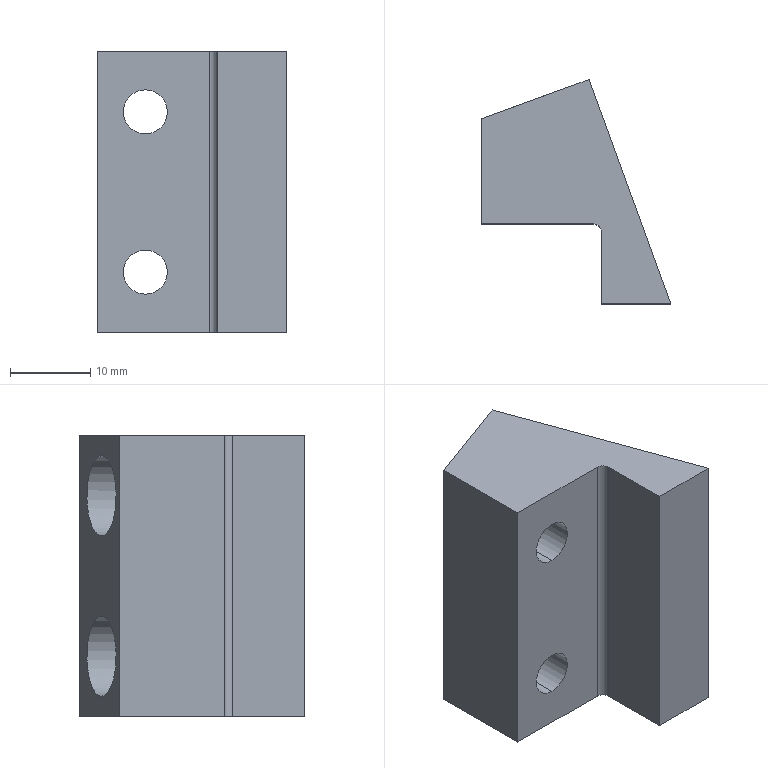Part | SolidWorks | features BaseBody 1 | 1 solid | 19 faces | box 23.64 x 28 x 35 mm | volume 9816 mm3 | plane 10 | cylinder 9 | commonest cylinder face diameters 5.5 x4 10 x4 2 x1
STEP:
#1=CARTESIAN_POINT('',(6.,4.,2.5));
#2=VERTEX_POINT('',#1);
#3=CARTESIAN_POINT('',(6.,4.,12.5));
#4=VERTEX_POINT('',#3);
#5=CARTESIAN_POINT('',(6.,4.,7.5));
#6=DIRECTION('',(0.,1.,0.));
#7=DIRECTION('',(0.,0.,1.));
#8=AXIS2_PLACEMENT_3D('',#5,#6,#7);
#9=CIRCLE('',#8,5.);
#10=EDGE_CURVE('',#2,#4,#9,.T.);
#11=ORIENTED_EDGE('',*,*,#10,.F.);
#12=CARTESIAN_POINT('',(6.,15.289,2.5));
#13=VERTEX_POINT('',#12);
#14=CARTESIAN_POINT('',(6.,18.,2.5));
#15=DIRECTION('',(0.,1.,0.));
#16=VECTOR('',#15,1000.);
#17=LINE('',#14,#16);
#18=EDGE_CURVE('',#2,#13,#17,.T.);
#19=ORIENTED_EDGE('',*,*,#18,.T.);
#20=CARTESIAN_POINT('',(6.,15.289,12.5));
#21=VERTEX_POINT('',#20);
#22=CARTESIAN_POINT('',(6.,15.289,2.5));
#23=CARTESIAN_POINT('',(-4.,11.649,2.5));
#24=CARTESIAN_POINT('',(-4.,11.649,12.5));
#25=CARTESIAN_POINT('',(6.,15.289,12.5));
#26=(BOUNDED_CURVE()B_SPLINE_CURVE(3,(#22,#23,#24,#25),.UNSPECIFIED.,.F.,.F.)B_SPLINE_CURVE_WITH_KNOTS((4,4),(1.571,4.712),.UNSPECIFIED.)CURVE()GEOMETRIC_REPRESENTATION_ITEM()RATIONAL_B_SPLINE_CURVE((1.,0.3333,0.3333,1.))REPRESENTATION_ITEM(''));
#27=EDGE_CURVE('',#13,#21,#26,.T.);
#28=ORIENTED_EDGE('',*,*,#27,.T.);
#29=CARTESIAN_POINT('',(6.,18.,12.5));
#30=DIRECTION('',(0.,1.,0.));
#31=VECTOR('',#30,1000.);
#32=LINE('',#29,#31);
#33=EDGE_CURVE('',#4,#21,#32,.T.);
#34=ORIENTED_EDGE('',*,*,#33,.F.);
#35=EDGE_LOOP('',(#11,#19,#28,#34));
#36=FACE_OUTER_BOUND('',#35,.T.);
#37=CARTESIAN_POINT('',(6.,18.,7.5));
#38=DIRECTION('',(0.,1.,0.));
#39=DIRECTION('',(0.,0.,1.));
#40=AXIS2_PLACEMENT_3D('',#37,#38,#39);
#41=CYLINDRICAL_SURFACE('',#40,5.);
#42=ADVANCED_FACE('',(#36),#41,.F.);
#43=CARTESIAN_POINT('',(6.,4.,22.5));
#44=VERTEX_POINT('',#43);
#45=CARTESIAN_POINT('',(6.,4.,32.5));
#46=VERTEX_POINT('',#45);
#47=CARTESIAN_POINT('',(6.,4.,27.5));
#48=DIRECTION('',(0.,1.,0.));
#49=DIRECTION('',(0.,0.,1.));
#50=AXIS2_PLACEMENT_3D('',#47,#48,#49);
#51=CIRCLE('',#50,5.);
#52=EDGE_CURVE('',#44,#46,#51,.T.);
#53=ORIENTED_EDGE('',*,*,#52,.F.);
#54=CARTESIAN_POINT('',(6.,15.289,22.5));
#55=VERTEX_POINT('',#54);
#56=CARTESIAN_POINT('',(6.,18.,22.5));
#57=DIRECTION('',(0.,1.,0.));
#58=VECTOR('',#57,1000.);
#59=LINE('',#56,#58);
#60=EDGE_CURVE('',#44,#55,#59,.T.);
#61=ORIENTED_EDGE('',*,*,#60,.T.);
#62=CARTESIAN_POINT('',(6.,15.289,32.5));
#63=VERTEX_POINT('',#62);
#64=CARTESIAN_POINT('',(6.,15.289,22.5));
#65=CARTESIAN_POINT('',(-4.,11.649,22.5));
#66=CARTESIAN_POINT('',(-4.,11.649,32.5));
#67=CARTESIAN_POINT('',(6.,15.289,32.5));
#68=(BOUNDED_CURVE()B_SPLINE_CURVE(3,(#64,#65,#66,#67),.UNSPECIFIED.,.F.,.T.)B_SPLINE_CURVE_WITH_KNOTS((4,4),(1.571,4.712),.UNSPECIFIED.)CURVE()GEOMETRIC_REPRESENTATION_ITEM()RATIONAL_B_SPLINE_CURVE((1.,0.3333,0.3333,1.))REPRESENTATION_ITEM(''));
#69=EDGE_CURVE('',#55,#63,#68,.T.);
#70=ORIENTED_EDGE('',*,*,#69,.T.);
#71=CARTESIAN_POINT('',(6.,18.,32.5));
#72=DIRECTION('',(0.,1.,0.));
#73=VECTOR('',#72,1000.);
#74=LINE('',#71,#73);
#75=EDGE_CURVE('',#46,#63,#74,.T.);
#76=ORIENTED_EDGE('',*,*,#75,.F.);
#77=EDGE_LOOP('',(#53,#61,#70,#76));
#78=FACE_OUTER_BOUND('',#77,.T.);
#79=CARTESIAN_POINT('',(6.,18.,27.5));
#80=DIRECTION('',(0.,1.,0.));
#81=DIRECTION('',(0.,0.,1.));
#82=AXIS2_PLACEMENT_3D('',#79,#80,#81);
#83=CYLINDRICAL_SURFACE('',#82,5.);
#84=ADVANCED_FACE('',(#78),#83,.F.);
#85=CARTESIAN_POINT('',(6.,0.,30.25));
#86=VERTEX_POINT('',#85);
#87=CARTESIAN_POINT('',(6.,0.,24.75));
#88=VERTEX_POINT('',#87);
#89=CARTESIAN_POINT('',(6.,0.,27.5));
#90=DIRECTION('',(0.,-1.,0.));
#91=DIRECTION('',(0.,0.,1.));
#92=AXIS2_PLACEMENT_3D('',#89,#90,#91);
#93=CIRCLE('',#92,2.75);
#94=EDGE_CURVE('',#86,#88,#93,.T.);
#95=ORIENTED_EDGE('',*,*,#94,.T.);
#96=CARTESIAN_POINT('',(6.,4.,24.75));
#97=VERTEX_POINT('',#96);
#98=CARTESIAN_POINT('',(6.,18.,24.75));
#99=DIRECTION('',(0.,1.,0.));
#100=VECTOR('',#99,1000.);
#101=LINE('',#98,#100);
#102=EDGE_CURVE('',#88,#97,#101,.T.);
#103=ORIENTED_EDGE('',*,*,#102,.T.);
#104=CARTESIAN_POINT('',(6.,4.,30.25));
#105=VERTEX_POINT('',#104);
#106=CARTESIAN_POINT('',(6.,4.,27.5));
#107=DIRECTION('',(0.,-1.,0.));
#108=DIRECTION('',(0.,0.,1.));
#109=AXIS2_PLACEMENT_3D('',#106,#107,#108);
#110=CIRCLE('',#109,2.75);
#111=EDGE_CURVE('',#105,#97,#110,.T.);
#112=ORIENTED_EDGE('',*,*,#111,.F.);
#113=CARTESIAN_POINT('',(6.,18.,30.25));
#114=DIRECTION('',(0.,1.,0.));
#115=VECTOR('',#114,1000.);
#116=LINE('',#113,#115);
#117=EDGE_CURVE('',#86,#105,#116,.T.);
#118=ORIENTED_EDGE('',*,*,#117,.F.);
#119=EDGE_LOOP('',(#95,#103,#112,#118));
#120=FACE_OUTER_BOUND('',#119,.T.);
#121=CARTESIAN_POINT('',(6.,18.,27.5));
#122=DIRECTION('',(0.,1.,0.));
#123=DIRECTION('',(0.,0.,1.));
#124=AXIS2_PLACEMENT_3D('',#121,#122,#123);
#125=CYLINDRICAL_SURFACE('',#124,2.75);
#126=ADVANCED_FACE('',(#120),#125,.F.);
#127=CARTESIAN_POINT('',(6.,0.,10.25));
#128=VERTEX_POINT('',#127);
#129=CARTESIAN_POINT('',(6.,0.,4.75));
#130=VERTEX_POINT('',#129);
#131=CARTESIAN_POINT('',(6.,0.,7.5));
#132=DIRECTION('',(0.,-1.,0.));
#133=DIRECTION('',(0.,0.,1.));
#134=AXIS2_PLACEMENT_3D('',#131,#132,#133);
#135=CIRCLE('',#134,2.75);
#136=EDGE_CURVE('',#128,#130,#135,.T.);
#137=ORIENTED_EDGE('',*,*,#136,.T.);
#138=CARTESIAN_POINT('',(6.,4.,4.75));
#139=VERTEX_POINT('',#138);
#140=CARTESIAN_POINT('',(6.,18.,4.75));
#141=DIRECTION('',(0.,1.,0.));
#142=VECTOR('',#141,1000.);
#143=LINE('',#140,#142);
#144=EDGE_CURVE('',#130,#139,#143,.T.);
#145=ORIENTED_EDGE('',*,*,#144,.T.);
#146=CARTESIAN_POINT('',(6.,4.,10.25));
#147=VERTEX_POINT('',#146);
#148=CARTESIAN_POINT('',(6.,4.,7.5));
#149=DIRECTION('',(0.,-1.,0.));
#150=DIRECTION('',(0.,0.,1.));
#151=AXIS2_PLACEMENT_3D('',#148,#149,#150);
#152=CIRCLE('',#151,2.75);
#153=EDGE_CURVE('',#147,#139,#152,.T.);
#154=ORIENTED_EDGE('',*,*,#153,.F.);
#155=CARTESIAN_POINT('',(6.,18.,10.25));
#156=DIRECTION('',(0.,1.,0.));
#157=VECTOR('',#156,1000.);
#158=LINE('',#155,#157);
#159=EDGE_CURVE('',#128,#147,#158,.T.);
#160=ORIENTED_EDGE('',*,*,#159,.F.);
#161=EDGE_LOOP('',(#137,#145,#154,#160));
#162=FACE_OUTER_BOUND('',#161,.T.);
#163=CARTESIAN_POINT('',(6.,18.,7.5));
#164=DIRECTION('',(0.,1.,0.));
#165=DIRECTION('',(0.,0.,1.));
#166=AXIS2_PLACEMENT_3D('',#163,#164,#165);
#167=CYLINDRICAL_SURFACE('',#166,2.75);
#168=ADVANCED_FACE('',(#162),#167,.F.);
#169=CARTESIAN_POINT('',(13.449,18.,35.));
#170=VERTEX_POINT('',#169);
#171=CARTESIAN_POINT('',(13.449,18.,0.));
#172=VERTEX_POINT('',#171);
#173=CARTESIAN_POINT('',(13.449,18.,35.));
#174=DIRECTION('',(0.,0.,-1.));
#175=VECTOR('',#174,1000.);
#176=LINE('',#173,#175);
#177=EDGE_CURVE('',#170,#172,#176,.T.);
#178=ORIENTED_EDGE('',*,*,#177,.F.);
#179=CARTESIAN_POINT('',(23.64,-10.,35.));
#180=VERTEX_POINT('',#179);
#181=CARTESIAN_POINT('',(13.449,18.,35.));
#182=DIRECTION('',(-0.342,0.9397,0.));
#183=VECTOR('',#182,1000.);
#184=LINE('',#181,#183);
#185=EDGE_CURVE('',#180,#170,#184,.T.);
#186=ORIENTED_EDGE('',*,*,#185,.F.);
#187=CARTESIAN_POINT('',(23.64,-10.,0.));
#188=VERTEX_POINT('',#187);
#189=CARTESIAN_POINT('',(23.64,-10.,35.));
#190=DIRECTION('',(0.,0.,1.));
#191=VECTOR('',#190,1000.);
#192=LINE('',#189,#191);
#193=EDGE_CURVE('',#188,#180,#192,.T.);
#194=ORIENTED_EDGE('',*,*,#193,.F.);
#195=CARTESIAN_POINT('',(13.449,18.,0.));
#196=DIRECTION('',(0.342,-0.9397,0.));
#197=VECTOR('',#196,1000.);
#198=LINE('',#195,#197);
#199=EDGE_CURVE('',#172,#188,#198,.T.);
#200=ORIENTED_EDGE('',*,*,#199,.F.);
#201=EDGE_LOOP('',(#178,#186,#194,#200));
#202=FACE_OUTER_BOUND('',#201,.T.);
#203=CARTESIAN_POINT('',(13.449,18.,35.));
#204=DIRECTION('',(-0.9397,-0.342,0.));
#205=DIRECTION('',(0.342,-0.9397,0.));
#206=AXIS2_PLACEMENT_3D('',#203,#204,#205);
#207=PLANE('',#206);
#208=ADVANCED_FACE('',(#202),#207,.F.);
#209=CARTESIAN_POINT('',(14.,0.,0.));
#210=VERTEX_POINT('',#209);
#211=CARTESIAN_POINT('',(0.,0.,0.));
#212=VERTEX_POINT('',#211);
#213=CARTESIAN_POINT('',(0.,0.,0.));
#214=DIRECTION('',(-1.,0.,0.));
#215=VECTOR('',#214,1000.);
#216=LINE('',#213,#215);
#217=EDGE_CURVE('',#210,#212,#216,.T.);
#218=ORIENTED_EDGE('',*,*,#217,.T.);
#219=CARTESIAN_POINT('',(0.,13.105,0.));
#220=VERTEX_POINT('',#219);
#221=CARTESIAN_POINT('',(0.,0.,0.));
#222=DIRECTION('',(0.,1.,0.));
#223=VECTOR('',#222,1000.);
#224=LINE('',#221,#223);
#225=EDGE_CURVE('',#212,#220,#224,.T.);
#226=ORIENTED_EDGE('',*,*,#225,.T.);
#227=CARTESIAN_POINT('',(0.,13.105,0.));
#228=DIRECTION('',(0.9397,0.342,0.));
#229=VECTOR('',#228,1000.);
#230=LINE('',#227,#229);
#231=EDGE_CURVE('',#220,#172,#230,.T.);
#232=ORIENTED_EDGE('',*,*,#231,.T.);
#233=ORIENTED_EDGE('',*,*,#199,.T.);
#234=CARTESIAN_POINT('',(15.,-10.,0.));
#235=VERTEX_POINT('',#234);
#236=CARTESIAN_POINT('',(0.,-10.,0.));
#237=DIRECTION('',(-1.,0.,0.));
#238=VECTOR('',#237,1000.);
#239=LINE('',#236,#238);
#240=EDGE_CURVE('',#188,#235,#239,.T.);
#241=ORIENTED_EDGE('',*,*,#240,.T.);
#242=CARTESIAN_POINT('',(15.,-1.,0.));
#243=VERTEX_POINT('',#242);
#244=CARTESIAN_POINT('',(15.,0.,0.));
#245=DIRECTION('',(0.,1.,0.));
#246=VECTOR('',#245,1000.);
#247=LINE('',#244,#246);
#248=EDGE_CURVE('',#235,#243,#247,.T.);
#249=ORIENTED_EDGE('',*,*,#248,.T.);
#250=CARTESIAN_POINT('',(14.,-1.,0.));
#251=DIRECTION('',(0.,0.,1.));
#252=DIRECTION('',(-1.,0.,0.));
#253=AXIS2_PLACEMENT_3D('',#250,#251,#252);
#254=CIRCLE('',#253,1.);
#255=EDGE_CURVE('',#243,#210,#254,.T.);
#256=ORIENTED_EDGE('',*,*,#255,.T.);
#257=EDGE_LOOP('',(#218,#226,#232,#233,#241,#249,#256));
#258=FACE_OUTER_BOUND('',#257,.T.);
#259=CARTESIAN_POINT('',(0.,0.,0.));
#260=DIRECTION('',(0.,0.,-1.));
#261=DIRECTION('',(-1.,0.,0.));
#262=AXIS2_PLACEMENT_3D('',#259,#260,#261);
#263=PLANE('',#262);
#264=ADVANCED_FACE('',(#258),#263,.T.);
#265=ORIENTED_EDGE('',*,*,#177,.T.);
#266=ORIENTED_EDGE('',*,*,#231,.F.);
#267=CARTESIAN_POINT('',(0.,13.105,35.));
#268=VERTEX_POINT('',#267);
#269=CARTESIAN_POINT('',(0.,13.105,35.));
#270=DIRECTION('',(0.,0.,-1.));
#271=VECTOR('',#270,1000.);
#272=LINE('',#269,#271);
#273=EDGE_CURVE('',#268,#220,#272,.T.);
#274=ORIENTED_EDGE('',*,*,#273,.F.);
#275=CARTESIAN_POINT('',(13.449,18.,35.));
#276=DIRECTION('',(-0.9397,-0.342,0.));
#277=VECTOR('',#276,1000.);
#278=LINE('',#275,#277);
#279=EDGE_CURVE('',#170,#268,#278,.T.);
#280=ORIENTED_EDGE('',*,*,#279,.F.);
#281=EDGE_LOOP('',(#265,#266,#274,#280));
#282=FACE_OUTER_BOUND('',#281,.T.);
#283=CARTESIAN_POINT('',(6.,15.289,12.5));
#284=CARTESIAN_POINT('',(16.,18.929,12.5));
#285=CARTESIAN_POINT('',(16.,18.929,2.5));
#286=CARTESIAN_POINT('',(6.,15.289,2.5));
#287=(BOUNDED_CURVE()B_SPLINE_CURVE(3,(#283,#284,#285,#286),.UNSPECIFIED.,.F.,.T.)B_SPLINE_CURVE_WITH_KNOTS((4,4),(4.712,7.854),.UNSPECIFIED.)CURVE()GEOMETRIC_REPRESENTATION_ITEM()RATIONAL_B_SPLINE_CURVE((1.,0.3333,0.3333,1.))REPRESENTATION_ITEM(''));
#288=EDGE_CURVE('',#21,#13,#287,.T.);
#289=ORIENTED_EDGE('',*,*,#288,.F.);
#290=ORIENTED_EDGE('',*,*,#27,.F.);
#291=EDGE_LOOP('',(#289,#290));
#292=FACE_BOUND('',#291,.T.);
#293=CARTESIAN_POINT('',(6.,15.289,32.5));
#294=CARTESIAN_POINT('',(16.,18.929,32.5));
#295=CARTESIAN_POINT('',(16.,18.929,22.5));
#296=CARTESIAN_POINT('',(6.,15.289,22.5));
#297=(BOUNDED_CURVE()B_SPLINE_CURVE(3,(#293,#294,#295,#296),.UNSPECIFIED.,.F.,.F.)B_SPLINE_CURVE_WITH_KNOTS((4,4),(4.712,7.854),.UNSPECIFIED.)CURVE()GEOMETRIC_REPRESENTATION_ITEM()RATIONAL_B_SPLINE_CURVE((1.,0.3333,0.3333,1.))REPRESENTATION_ITEM(''));
#298=EDGE_CURVE('',#63,#55,#297,.T.);
#299=ORIENTED_EDGE('',*,*,#298,.F.);
#300=ORIENTED_EDGE('',*,*,#69,.F.);
#301=EDGE_LOOP('',(#299,#300));
#302=FACE_BOUND('',#301,.T.);
#303=CARTESIAN_POINT('',(13.449,18.,35.));
#304=DIRECTION('',(0.342,-0.9397,0.));
#305=DIRECTION('',(0.9397,0.342,0.));
#306=AXIS2_PLACEMENT_3D('',#303,#304,#305);
#307=PLANE('',#306);
#308=ADVANCED_FACE('',(#282,#292,#302),#307,.F.);
#309=ORIENTED_EDGE('',*,*,#279,.T.);
#310=CARTESIAN_POINT('',(0.,0.,35.));
#311=VERTEX_POINT('',#310);
#312=CARTESIAN_POINT('',(0.,0.,35.));
#313=DIRECTION('',(0.,1.,0.));
#314=VECTOR('',#313,1000.);
#315=LINE('',#312,#314);
#316=EDGE_CURVE('',#311,#268,#315,.T.);
#317=ORIENTED_EDGE('',*,*,#316,.F.);
#318=CARTESIAN_POINT('',(14.,0.,35.));
#319=VERTEX_POINT('',#318);
#320=CARTESIAN_POINT('',(0.,0.,35.));
#321=DIRECTION('',(-1.,0.,0.));
#322=VECTOR('',#321,1000.);
#323=LINE('',#320,#322);
#324=EDGE_CURVE('',#319,#311,#323,.T.);
#325=ORIENTED_EDGE('',*,*,#324,.F.);
#326=CARTESIAN_POINT('',(15.,-1.,35.));
#327=VERTEX_POINT('',#326);
#328=CARTESIAN_POINT('',(14.,-1.,35.));
#329=DIRECTION('',(0.,0.,-1.));
#330=DIRECTION('',(-1.,0.,0.));
#331=AXIS2_PLACEMENT_3D('',#328,#329,#330);
#332=CIRCLE('',#331,1.);
#333=EDGE_CURVE('',#319,#327,#332,.T.);
#334=ORIENTED_EDGE('',*,*,#333,.T.);
#335=CARTESIAN_POINT('',(15.,-10.,35.));
#336=VERTEX_POINT('',#335);
#337=CARTESIAN_POINT('',(15.,0.,35.));
#338=DIRECTION('',(0.,1.,0.));
#339=VECTOR('',#338,1000.);
#340=LINE('',#337,#339);
#341=EDGE_CURVE('',#336,#327,#340,.T.);
#342=ORIENTED_EDGE('',*,*,#341,.F.);
#343=CARTESIAN_POINT('',(0.,-10.,35.));
#344=DIRECTION('',(-1.,0.,0.));
#345=VECTOR('',#344,1000.);
#346=LINE('',#343,#345);
#347=EDGE_CURVE('',#180,#336,#346,.T.);
#348=ORIENTED_EDGE('',*,*,#347,.F.);
#349=ORIENTED_EDGE('',*,*,#185,.T.);
#350=EDGE_LOOP('',(#309,#317,#325,#334,#342,#348,#349));
#351=FACE_OUTER_BOUND('',#350,.T.);
#352=CARTESIAN_POINT('',(0.,0.,35.));
#353=DIRECTION('',(0.,0.,-1.));
#354=DIRECTION('',(-1.,0.,0.));
#355=AXIS2_PLACEMENT_3D('',#352,#353,#354);
#356=PLANE('',#355);
#357=ADVANCED_FACE('',(#351),#356,.F.);
#358=ORIENTED_EDGE('',*,*,#347,.T.);
#359=CARTESIAN_POINT('',(15.,-10.,35.));
#360=DIRECTION('',(0.,0.,-1.));
#361=VECTOR('',#360,1000.);
#362=LINE('',#359,#361);
#363=EDGE_CURVE('',#336,#235,#362,.T.);
#364=ORIENTED_EDGE('',*,*,#363,.T.);
#365=ORIENTED_EDGE('',*,*,#240,.F.);
#366=ORIENTED_EDGE('',*,*,#193,.T.);
#367=EDGE_LOOP('',(#358,#364,#365,#366));
#368=FACE_OUTER_BOUND('',#367,.T.);
#369=CARTESIAN_POINT('',(15.,-10.,35.));
#370=DIRECTION('',(0.,-1.,0.));
#371=DIRECTION('',(0.,0.,-1.));
#372=AXIS2_PLACEMENT_3D('',#369,#370,#371);
#373=PLANE('',#372);
#374=ADVANCED_FACE('',(#368),#373,.T.);
#375=ORIENTED_EDGE('',*,*,#273,.T.);
#376=ORIENTED_EDGE('',*,*,#225,.F.);
#377=CARTESIAN_POINT('',(0.,0.,35.));
#378=DIRECTION('',(0.,0.,-1.));
#379=VECTOR('',#378,1000.);
#380=LINE('',#377,#379);
#381=EDGE_CURVE('',#311,#212,#380,.T.);
#382=ORIENTED_EDGE('',*,*,#381,.F.);
#383=ORIENTED_EDGE('',*,*,#316,.T.);
#384=EDGE_LOOP('',(#375,#376,#382,#383));
#385=FACE_OUTER_BOUND('',#384,.T.);
#386=CARTESIAN_POINT('',(0.,0.,35.));
#387=DIRECTION('',(1.,0.,0.));
#388=DIRECTION('',(0.,0.,-1.));
#389=AXIS2_PLACEMENT_3D('',#386,#387,#388);
#390=PLANE('',#389);
#391=ADVANCED_FACE('',(#385),#390,.F.);
#392=CARTESIAN_POINT('',(14.,0.,35.));
#393=DIRECTION('',(0.,0.,-1.));
#394=VECTOR('',#393,1000.);
#395=LINE('',#392,#394);
#396=EDGE_CURVE('',#319,#210,#395,.T.);
#397=ORIENTED_EDGE('',*,*,#396,.F.);
#398=ORIENTED_EDGE('',*,*,#324,.T.);
#399=ORIENTED_EDGE('',*,*,#381,.T.);
#400=ORIENTED_EDGE('',*,*,#217,.F.);
#401=EDGE_LOOP('',(#397,#398,#399,#400));
#402=FACE_OUTER_BOUND('',#401,.T.);
#403=ORIENTED_EDGE('',*,*,#94,.F.);
#404=CARTESIAN_POINT('',(6.,0.,27.5));
#405=DIRECTION('',(0.,-1.,0.));
#406=DIRECTION('',(0.,0.,1.));
#407=AXIS2_PLACEMENT_3D('',#404,#405,#406);
#408=CIRCLE('',#407,2.75);
#409=EDGE_CURVE('',#88,#86,#408,.T.);
#410=ORIENTED_EDGE('',*,*,#409,.F.);
#411=EDGE_LOOP('',(#403,#410));
#412=FACE_BOUND('',#411,.T.);
#413=ORIENTED_EDGE('',*,*,#136,.F.);
#414=CARTESIAN_POINT('',(6.,0.,7.5));
#415=DIRECTION('',(0.,-1.,0.));
#416=DIRECTION('',(0.,0.,1.));
#417=AXIS2_PLACEMENT_3D('',#414,#415,#416);
#418=CIRCLE('',#417,2.75);
#419=EDGE_CURVE('',#130,#128,#418,.T.);
#420=ORIENTED_EDGE('',*,*,#419,.F.);
#421=EDGE_LOOP('',(#413,#420));
#422=FACE_BOUND('',#421,.T.);
#423=CARTESIAN_POINT('',(0.,0.,35.));
#424=DIRECTION('',(0.,1.,0.));
#425=DIRECTION('',(0.,0.,1.));
#426=AXIS2_PLACEMENT_3D('',#423,#424,#425);
#427=PLANE('',#426);
#428=ADVANCED_FACE('',(#402,#412,#422),#427,.F.);
#429=ORIENTED_EDGE('',*,*,#248,.F.);
#430=ORIENTED_EDGE('',*,*,#363,.F.);
#431=ORIENTED_EDGE('',*,*,#341,.T.);
#432=CARTESIAN_POINT('',(15.,-1.,35.));
#433=DIRECTION('',(0.,0.,-1.));
#434=VECTOR('',#433,1000.);
#435=LINE('',#432,#434);
#436=EDGE_CURVE('',#327,#243,#435,.T.);
#437=ORIENTED_EDGE('',*,*,#436,.T.);
#438=EDGE_LOOP('',(#429,#430,#431,#437));
#439=FACE_OUTER_BOUND('',#438,.T.);
#440=CARTESIAN_POINT('',(15.,0.,35.));
#441=DIRECTION('',(-1.,0.,0.));
#442=DIRECTION('',(0.,-1.,0.));
#443=AXIS2_PLACEMENT_3D('',#440,#441,#442);
#444=PLANE('',#443);
#445=ADVANCED_FACE('',(#439),#444,.T.);
#446=ORIENTED_EDGE('',*,*,#18,.F.);
#447=CARTESIAN_POINT('',(6.,4.,7.5));
#448=DIRECTION('',(0.,1.,0.));
#449=DIRECTION('',(0.,0.,1.));
#450=AXIS2_PLACEMENT_3D('',#447,#448,#449);
#451=CIRCLE('',#450,5.);
#452=EDGE_CURVE('',#4,#2,#451,.T.);
#453=ORIENTED_EDGE('',*,*,#452,.F.);
#454=ORIENTED_EDGE('',*,*,#33,.T.);
#455=ORIENTED_EDGE('',*,*,#288,.T.);
#456=EDGE_LOOP('',(#446,#453,#454,#455));
#457=FACE_OUTER_BOUND('',#456,.T.);
#458=CARTESIAN_POINT('',(6.,18.,7.5));
#459=DIRECTION('',(0.,1.,0.));
#460=DIRECTION('',(0.,0.,1.));
#461=AXIS2_PLACEMENT_3D('',#458,#459,#460);
#462=CYLINDRICAL_SURFACE('',#461,5.);
#463=ADVANCED_FACE('',(#457),#462,.F.);
#464=ORIENTED_EDGE('',*,*,#60,.F.);
#465=CARTESIAN_POINT('',(6.,4.,27.5));
#466=DIRECTION('',(0.,1.,0.));
#467=DIRECTION('',(0.,0.,1.));
#468=AXIS2_PLACEMENT_3D('',#465,#466,#467);
#469=CIRCLE('',#468,5.);
#470=EDGE_CURVE('',#46,#44,#469,.T.);
#471=ORIENTED_EDGE('',*,*,#470,.F.);
#472=ORIENTED_EDGE('',*,*,#75,.T.);
#473=ORIENTED_EDGE('',*,*,#298,.T.);
#474=EDGE_LOOP('',(#464,#471,#472,#473));
#475=FACE_OUTER_BOUND('',#474,.T.);
#476=CARTESIAN_POINT('',(6.,18.,27.5));
#477=DIRECTION('',(0.,1.,0.));
#478=DIRECTION('',(0.,0.,1.));
#479=AXIS2_PLACEMENT_3D('',#476,#477,#478);
#480=CYLINDRICAL_SURFACE('',#479,5.);
#481=ADVANCED_FACE('',(#475),#480,.F.);
#482=ORIENTED_EDGE('',*,*,#396,.T.);
#483=ORIENTED_EDGE('',*,*,#255,.F.);
#484=ORIENTED_EDGE('',*,*,#436,.F.);
#485=ORIENTED_EDGE('',*,*,#333,.F.);
#486=EDGE_LOOP('',(#482,#483,#484,#485));
#487=FACE_OUTER_BOUND('',#486,.T.);
#488=CARTESIAN_POINT('',(14.,-1.,35.));
#489=DIRECTION('',(0.,0.,-1.));
#490=DIRECTION('',(-1.,0.,0.));
#491=AXIS2_PLACEMENT_3D('',#488,#489,#490);
#492=CYLINDRICAL_SURFACE('',#491,1.);
#493=ADVANCED_FACE('',(#487),#492,.F.);
#494=ORIENTED_EDGE('',*,*,#102,.F.);
#495=ORIENTED_EDGE('',*,*,#409,.T.);
#496=ORIENTED_EDGE('',*,*,#117,.T.);
#497=CARTESIAN_POINT('',(6.,4.,27.5));
#498=DIRECTION('',(0.,-1.,0.));
#499=DIRECTION('',(0.,0.,1.));
#500=AXIS2_PLACEMENT_3D('',#497,#498,#499);
#501=CIRCLE('',#500,2.75);
#502=EDGE_CURVE('',#97,#105,#501,.T.);
#503=ORIENTED_EDGE('',*,*,#502,.F.);
#504=EDGE_LOOP('',(#494,#495,#496,#503));
#505=FACE_OUTER_BOUND('',#504,.T.);
#506=CARTESIAN_POINT('',(6.,18.,27.5));
#507=DIRECTION('',(0.,1.,0.));
#508=DIRECTION('',(0.,0.,1.));
#509=AXIS2_PLACEMENT_3D('',#506,#507,#508);
#510=CYLINDRICAL_SURFACE('',#509,2.75);
#511=ADVANCED_FACE('',(#505),#510,.F.);
#512=ORIENTED_EDGE('',*,*,#144,.F.);
#513=ORIENTED_EDGE('',*,*,#419,.T.);
#514=ORIENTED_EDGE('',*,*,#159,.T.);
#515=CARTESIAN_POINT('',(6.,4.,7.5));
#516=DIRECTION('',(0.,-1.,0.));
#517=DIRECTION('',(0.,0.,1.));
#518=AXIS2_PLACEMENT_3D('',#515,#516,#517);
#519=CIRCLE('',#518,2.75);
#520=EDGE_CURVE('',#139,#147,#519,.T.);
#521=ORIENTED_EDGE('',*,*,#520,.F.);
#522=EDGE_LOOP('',(#512,#513,#514,#521));
#523=FACE_OUTER_BOUND('',#522,.T.);
#524=CARTESIAN_POINT('',(6.,18.,7.5));
#525=DIRECTION('',(0.,1.,0.));
#526=DIRECTION('',(0.,0.,1.));
#527=AXIS2_PLACEMENT_3D('',#524,#525,#526);
#528=CYLINDRICAL_SURFACE('',#527,2.75);
#529=ADVANCED_FACE('',(#523),#528,.F.);
#530=ORIENTED_EDGE('',*,*,#452,.T.);
#531=ORIENTED_EDGE('',*,*,#10,.T.);
#532=EDGE_LOOP('',(#530,#531));
#533=FACE_OUTER_BOUND('',#532,.T.);
#534=ORIENTED_EDGE('',*,*,#153,.T.);
#535=ORIENTED_EDGE('',*,*,#520,.T.);
#536=EDGE_LOOP('',(#534,#535));
#537=FACE_BOUND('',#536,.T.);
#538=CARTESIAN_POINT('',(8.75,4.,7.5));
#539=DIRECTION('',(0.,-1.,0.));
#540=DIRECTION('',(0.,0.,-1.));
#541=AXIS2_PLACEMENT_3D('',#538,#539,#540);
#542=PLANE('',#541);
#543=ADVANCED_FACE('',(#533,#537),#542,.F.);
#544=ORIENTED_EDGE('',*,*,#470,.T.);
#545=ORIENTED_EDGE('',*,*,#52,.T.);
#546=EDGE_LOOP('',(#544,#545));
#547=FACE_OUTER_BOUND('',#546,.T.);
#548=ORIENTED_EDGE('',*,*,#111,.T.);
#549=ORIENTED_EDGE('',*,*,#502,.T.);
#550=EDGE_LOOP('',(#548,#549));
#551=FACE_BOUND('',#550,.T.);
#552=CARTESIAN_POINT('',(8.75,4.,27.5));
#553=DIRECTION('',(0.,-1.,0.));
#554=DIRECTION('',(0.,0.,-1.));
#555=AXIS2_PLACEMENT_3D('',#552,#553,#554);
#556=PLANE('',#555);
#557=ADVANCED_FACE('',(#547,#551),#556,.F.);
#558=CLOSED_SHELL('',(#42,#84,#126,#168,#208,#264,#308,#357,#374,#391,#428,#445,#463,#481,#493,#511,#529,#543,#557));
#559=MANIFOLD_SOLID_BREP('',#558);
#560=CARTESIAN_POINT('',(0.,0.,0.));
#561=DIRECTION('',(0.,0.,1.));
#562=DIRECTION('',(1.,0.,0.));
#563=AXIS2_PLACEMENT_3D('',#560,#561,#562);
#564=(LENGTH_UNIT()NAMED_UNIT(*)SI_UNIT(.MILLI.,.METRE.));
#565=UNCERTAINTY_MEASURE_WITH_UNIT(LENGTH_MEASURE(0.00001),#564,'','');
#566=(NAMED_UNIT(*)PLANE_ANGLE_UNIT()SI_UNIT($,.RADIAN.));
#567=(NAMED_UNIT(*)SI_UNIT($,.STERADIAN.)SOLID_ANGLE_UNIT());
#568=(GEOMETRIC_REPRESENTATION_CONTEXT(3)GLOBAL_UNCERTAINTY_ASSIGNED_CONTEXT((#565))GLOBAL_UNIT_ASSIGNED_CONTEXT((#564,#566,#567))REPRESENTATION_CONTEXT('',''));
#569=ADVANCED_BREP_SHAPE_REPRESENTATION('',(#559,#563),#568);